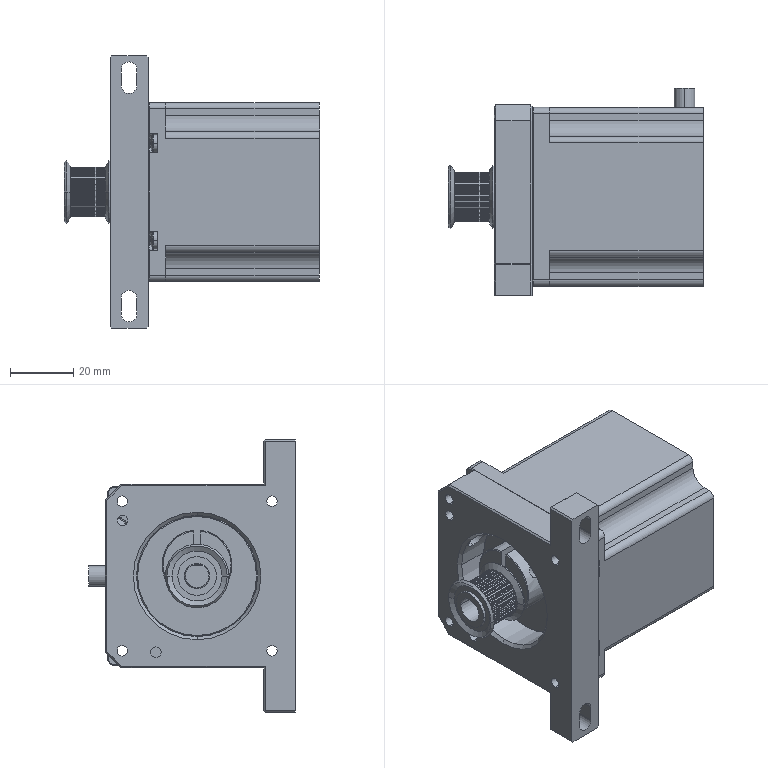Part | NX | features BREP 4 | 4 solids | 2187 faces | box 80.7 x 65.2 x 86 mm | volume 191758 mm3 | plane 1361 | spline 428 | cylinder 311 | cone 75 | torus 8 | sphere 4 | commonest cylinder face diameters 0.46 x120 15.66 x25 3.3 x14 5 x14 4 x12 2.5 x8